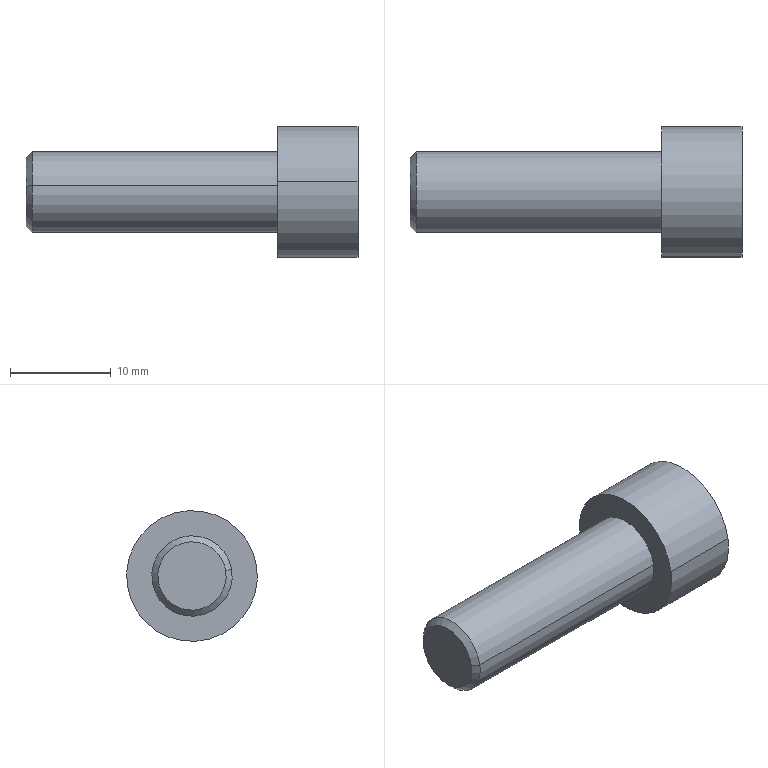Part | SolidWorks | features BaseBody 1 | 1 solid | 16 faces | box 33 x 13 x 13 mm | volume 2189 mm3 | plane 10 | cylinder 4 | cone 2 | commonest cylinder face diameters 8 x2 13 x2
STEP:
#1=CARTESIAN_POINT('',(251.6,-33.855,-27.446));
#2=VERTEX_POINT('',#1);
#3=CARTESIAN_POINT('',(251.6,-27.145,-28.554));
#4=VERTEX_POINT('',#3);
#5=CARTESIAN_POINT('',(251.6,-30.5,-28.));
#6=DIRECTION('',(-1.,0.,0.));
#7=DIRECTION('',(0.,-0.9866,0.1629));
#8=AXIS2_PLACEMENT_3D('',#5,#6,#7);
#9=CIRCLE('',#8,3.4);
#10=EDGE_CURVE('',#2,#4,#9,.T.);
#11=ORIENTED_EDGE('',*,*,#10,.F.);
#12=CARTESIAN_POINT('',(252.2,-34.447,-27.348));
#13=VERTEX_POINT('',#12);
#14=CARTESIAN_POINT('',(251.6,-33.855,-27.446));
#15=DIRECTION('',(0.7071,-0.6977,0.1152));
#16=VECTOR('',#15,1000.);
#17=LINE('',#14,#16);
#18=EDGE_CURVE('',#2,#13,#17,.T.);
#19=ORIENTED_EDGE('',*,*,#18,.T.);
#20=CARTESIAN_POINT('',(252.2,-26.553,-28.652));
#21=VERTEX_POINT('',#20);
#22=CARTESIAN_POINT('',(252.2,-30.5,-28.));
#23=DIRECTION('',(1.,0.,0.));
#24=DIRECTION('',(0.,-0.9866,0.1629));
#25=AXIS2_PLACEMENT_3D('',#22,#23,#24);
#26=CIRCLE('',#25,4.);
#27=EDGE_CURVE('',#21,#13,#26,.T.);
#28=ORIENTED_EDGE('',*,*,#27,.F.);
#29=CARTESIAN_POINT('',(251.6,-27.145,-28.554));
#30=DIRECTION('',(0.7071,0.6977,-0.1152));
#31=VECTOR('',#30,1000.);
#32=LINE('',#29,#31);
#33=EDGE_CURVE('',#4,#21,#32,.T.);
#34=ORIENTED_EDGE('',*,*,#33,.F.);
#35=EDGE_LOOP('',(#11,#19,#28,#34));
#36=FACE_OUTER_BOUND('',#35,.T.);
#37=CARTESIAN_POINT('',(251.6,-30.5,-28.));
#38=DIRECTION('',(1.,0.,0.));
#39=DIRECTION('',(0.,0.9866,-0.1629));
#40=AXIS2_PLACEMENT_3D('',#37,#38,#39);
#41=CONICAL_SURFACE('',#40,3.4,0.7854);
#42=ADVANCED_FACE('',(#36),#41,.T.);
#43=ORIENTED_EDGE('',*,*,#27,.T.);
#44=CARTESIAN_POINT('',(276.6,-34.447,-27.348));
#45=VERTEX_POINT('',#44);
#46=CARTESIAN_POINT('',(251.6,-34.447,-27.348));
#47=DIRECTION('',(1.,0.,0.));
#48=VECTOR('',#47,1000.);
#49=LINE('',#46,#48);
#50=EDGE_CURVE('',#13,#45,#49,.T.);
#51=ORIENTED_EDGE('',*,*,#50,.T.);
#52=CARTESIAN_POINT('',(276.6,-26.553,-28.652));
#53=VERTEX_POINT('',#52);
#54=CARTESIAN_POINT('',(276.6,-30.5,-28.));
#55=DIRECTION('',(-1.,0.,0.));
#56=DIRECTION('',(0.,-0.9866,0.1629));
#57=AXIS2_PLACEMENT_3D('',#54,#55,#56);
#58=CIRCLE('',#57,4.);
#59=EDGE_CURVE('',#45,#53,#58,.T.);
#60=ORIENTED_EDGE('',*,*,#59,.T.);
#61=CARTESIAN_POINT('',(251.6,-26.553,-28.652));
#62=DIRECTION('',(1.,0.,0.));
#63=VECTOR('',#62,1000.);
#64=LINE('',#61,#63);
#65=EDGE_CURVE('',#21,#53,#64,.T.);
#66=ORIENTED_EDGE('',*,*,#65,.F.);
#67=EDGE_LOOP('',(#43,#51,#60,#66));
#68=FACE_OUTER_BOUND('',#67,.T.);
#69=CARTESIAN_POINT('',(251.6,-30.5,-28.));
#70=DIRECTION('',(1.,0.,0.));
#71=DIRECTION('',(0.,0.9866,-0.1629));
#72=AXIS2_PLACEMENT_3D('',#69,#70,#71);
#73=CYLINDRICAL_SURFACE('',#72,4.);
#74=ADVANCED_FACE('',(#68),#73,.T.);
#75=CARTESIAN_POINT('',(276.6,-36.913,-26.941));
#76=VERTEX_POINT('',#75);
#77=CARTESIAN_POINT('',(276.6,-24.087,-29.059));
#78=VERTEX_POINT('',#77);
#79=CARTESIAN_POINT('',(276.6,-30.5,-28.));
#80=DIRECTION('',(-1.,0.,0.));
#81=DIRECTION('',(0.,-0.9866,0.1629));
#82=AXIS2_PLACEMENT_3D('',#79,#80,#81);
#83=CIRCLE('',#82,6.5);
#84=EDGE_CURVE('',#76,#78,#83,.T.);
#85=ORIENTED_EDGE('',*,*,#84,.F.);
#86=CARTESIAN_POINT('',(284.6,-36.913,-26.941));
#87=VERTEX_POINT('',#86);
#88=CARTESIAN_POINT('',(276.6,-36.913,-26.941));
#89=DIRECTION('',(1.,0.,0.));
#90=VECTOR('',#89,1000.);
#91=LINE('',#88,#90);
#92=EDGE_CURVE('',#76,#87,#91,.T.);
#93=ORIENTED_EDGE('',*,*,#92,.T.);
#94=CARTESIAN_POINT('',(284.6,-24.087,-29.059));
#95=VERTEX_POINT('',#94);
#96=CARTESIAN_POINT('',(284.6,-30.5,-28.));
#97=DIRECTION('',(-1.,0.,0.));
#98=DIRECTION('',(0.,-0.9866,0.1629));
#99=AXIS2_PLACEMENT_3D('',#96,#97,#98);
#100=CIRCLE('',#99,6.5);
#101=EDGE_CURVE('',#87,#95,#100,.T.);
#102=ORIENTED_EDGE('',*,*,#101,.T.);
#103=CARTESIAN_POINT('',(276.6,-24.087,-29.059));
#104=DIRECTION('',(1.,0.,0.));
#105=VECTOR('',#104,1000.);
#106=LINE('',#103,#105);
#107=EDGE_CURVE('',#78,#95,#106,.T.);
#108=ORIENTED_EDGE('',*,*,#107,.F.);
#109=EDGE_LOOP('',(#85,#93,#102,#108));
#110=FACE_OUTER_BOUND('',#109,.T.);
#111=CARTESIAN_POINT('',(276.6,-30.5,-28.));
#112=DIRECTION('',(1.,0.,0.));
#113=DIRECTION('',(0.,0.9866,-0.1629));
#114=AXIS2_PLACEMENT_3D('',#111,#112,#113);
#115=CYLINDRICAL_SURFACE('',#114,6.5);
#116=ADVANCED_FACE('',(#110),#115,.T.);
#117=CARTESIAN_POINT('',(276.6,-30.5,-28.));
#118=DIRECTION('',(-1.,0.,0.));
#119=DIRECTION('',(0.,-0.9866,0.1629));
#120=AXIS2_PLACEMENT_3D('',#117,#118,#119);
#121=CIRCLE('',#120,6.5);
#122=EDGE_CURVE('',#78,#76,#121,.T.);
#123=ORIENTED_EDGE('',*,*,#122,.T.);
#124=ORIENTED_EDGE('',*,*,#84,.T.);
#125=EDGE_LOOP('',(#123,#124));
#126=FACE_OUTER_BOUND('',#125,.T.);
#127=CARTESIAN_POINT('',(276.6,-30.5,-28.));
#128=DIRECTION('',(-1.,0.,0.));
#129=DIRECTION('',(0.,-0.9866,0.1629));
#130=AXIS2_PLACEMENT_3D('',#127,#128,#129);
#131=CIRCLE('',#130,4.);
#132=EDGE_CURVE('',#53,#45,#131,.T.);
#133=ORIENTED_EDGE('',*,*,#132,.F.);
#134=ORIENTED_EDGE('',*,*,#59,.F.);
#135=EDGE_LOOP('',(#133,#134));
#136=FACE_BOUND('',#135,.T.);
#137=CARTESIAN_POINT('',(276.6,-30.5,-28.));
#138=DIRECTION('',(-1.,0.,0.));
#139=DIRECTION('',(0.,-0.9866,0.1629));
#140=AXIS2_PLACEMENT_3D('',#137,#138,#139);
#141=PLANE('',#140);
#142=ADVANCED_FACE('',(#126,#136),#141,.T.);
#143=ORIENTED_EDGE('',*,*,#92,.F.);
#144=ORIENTED_EDGE('',*,*,#122,.F.);
#145=ORIENTED_EDGE('',*,*,#107,.T.);
#146=CARTESIAN_POINT('',(284.6,-30.5,-28.));
#147=DIRECTION('',(-1.,0.,0.));
#148=DIRECTION('',(0.,-0.9866,0.1629));
#149=AXIS2_PLACEMENT_3D('',#146,#147,#148);
#150=CIRCLE('',#149,6.5);
#151=EDGE_CURVE('',#95,#87,#150,.T.);
#152=ORIENTED_EDGE('',*,*,#151,.T.);
#153=EDGE_LOOP('',(#143,#144,#145,#152));
#154=FACE_OUTER_BOUND('',#153,.T.);
#155=CARTESIAN_POINT('',(276.6,-30.5,-28.));
#156=DIRECTION('',(1.,0.,0.));
#157=DIRECTION('',(0.,0.9866,-0.1629));
#158=AXIS2_PLACEMENT_3D('',#155,#156,#157);
#159=CYLINDRICAL_SURFACE('',#158,6.5);
#160=ADVANCED_FACE('',(#154),#159,.T.);
#161=CARTESIAN_POINT('',(284.6,-33.178,-25.802));
#162=VERTEX_POINT('',#161);
#163=CARTESIAN_POINT('',(284.6,-33.742,-29.22));
#164=VERTEX_POINT('',#163);
#165=CARTESIAN_POINT('',(284.6,-33.178,-25.802));
#166=DIRECTION('',(0.,-0.1629,-0.9866));
#167=VECTOR('',#166,1000.);
#168=LINE('',#165,#167);
#169=EDGE_CURVE('',#162,#164,#168,.T.);
#170=ORIENTED_EDGE('',*,*,#169,.F.);
#171=CARTESIAN_POINT('',(284.6,-29.936,-24.582));
#172=VERTEX_POINT('',#171);
#173=CARTESIAN_POINT('',(284.6,-29.936,-24.582));
#174=DIRECTION('',(0.,-0.9359,-0.3522));
#175=VECTOR('',#174,1000.);
#176=LINE('',#173,#175);
#177=EDGE_CURVE('',#172,#162,#176,.T.);
#178=ORIENTED_EDGE('',*,*,#177,.F.);
#179=CARTESIAN_POINT('',(284.6,-27.258,-26.78));
#180=VERTEX_POINT('',#179);
#181=CARTESIAN_POINT('',(284.6,-29.936,-24.582));
#182=DIRECTION('',(0.,-0.773,0.6344));
#183=VECTOR('',#182,1000.);
#184=LINE('',#181,#183);
#185=EDGE_CURVE('',#180,#172,#184,.T.);
#186=ORIENTED_EDGE('',*,*,#185,.F.);
#187=CARTESIAN_POINT('',(284.6,-27.822,-30.198));
#188=VERTEX_POINT('',#187);
#189=CARTESIAN_POINT('',(284.6,-27.258,-26.78));
#190=DIRECTION('',(0.,0.1629,0.9866));
#191=VECTOR('',#190,1000.);
#192=LINE('',#189,#191);
#193=EDGE_CURVE('',#188,#180,#192,.T.);
#194=ORIENTED_EDGE('',*,*,#193,.F.);
#195=CARTESIAN_POINT('',(284.6,-31.064,-31.418));
#196=VERTEX_POINT('',#195);
#197=CARTESIAN_POINT('',(284.6,-31.064,-31.418));
#198=DIRECTION('',(0.,0.9359,0.3522));
#199=VECTOR('',#198,1000.);
#200=LINE('',#197,#199);
#201=EDGE_CURVE('',#196,#188,#200,.T.);
#202=ORIENTED_EDGE('',*,*,#201,.F.);
#203=CARTESIAN_POINT('',(284.6,-31.064,-31.418));
#204=DIRECTION('',(0.,0.773,-0.6344));
#205=VECTOR('',#204,1000.);
#206=LINE('',#203,#205);
#207=EDGE_CURVE('',#164,#196,#206,.T.);
#208=ORIENTED_EDGE('',*,*,#207,.F.);
#209=EDGE_LOOP('',(#170,#178,#186,#194,#202,#208));
#210=FACE_BOUND('',#209,.T.);
#211=ORIENTED_EDGE('',*,*,#151,.F.);
#212=ORIENTED_EDGE('',*,*,#101,.F.);
#213=EDGE_LOOP('',(#211,#212));
#214=FACE_OUTER_BOUND('',#213,.T.);
#215=CARTESIAN_POINT('',(284.6,-30.5,-28.));
#216=DIRECTION('',(-1.,0.,0.));
#217=DIRECTION('',(0.,-0.9866,0.1629));
#218=AXIS2_PLACEMENT_3D('',#215,#216,#217);
#219=PLANE('',#218);
#220=ADVANCED_FACE('',(#210,#214),#219,.F.);
#221=ORIENTED_EDGE('',*,*,#50,.F.);
#222=CARTESIAN_POINT('',(252.2,-30.5,-28.));
#223=DIRECTION('',(1.,0.,0.));
#224=DIRECTION('',(0.,-0.9866,0.1629));
#225=AXIS2_PLACEMENT_3D('',#222,#223,#224);
#226=CIRCLE('',#225,4.);
#227=EDGE_CURVE('',#13,#21,#226,.T.);
#228=ORIENTED_EDGE('',*,*,#227,.T.);
#229=ORIENTED_EDGE('',*,*,#65,.T.);
#230=ORIENTED_EDGE('',*,*,#132,.T.);
#231=EDGE_LOOP('',(#221,#228,#229,#230));
#232=FACE_OUTER_BOUND('',#231,.T.);
#233=CARTESIAN_POINT('',(251.6,-30.5,-28.));
#234=DIRECTION('',(1.,0.,0.));
#235=DIRECTION('',(0.,0.9866,-0.1629));
#236=AXIS2_PLACEMENT_3D('',#233,#234,#235);
#237=CYLINDRICAL_SURFACE('',#236,4.);
#238=ADVANCED_FACE('',(#232),#237,.T.);
#239=CARTESIAN_POINT('',(251.6,-30.5,-28.));
#240=DIRECTION('',(-1.,0.,0.));
#241=DIRECTION('',(0.,-0.9866,0.1629));
#242=AXIS2_PLACEMENT_3D('',#239,#240,#241);
#243=CIRCLE('',#242,3.4);
#244=EDGE_CURVE('',#4,#2,#243,.T.);
#245=ORIENTED_EDGE('',*,*,#244,.T.);
#246=ORIENTED_EDGE('',*,*,#10,.T.);
#247=EDGE_LOOP('',(#245,#246));
#248=FACE_OUTER_BOUND('',#247,.T.);
#249=CARTESIAN_POINT('',(251.6,-30.5,-28.));
#250=DIRECTION('',(-1.,0.,0.));
#251=DIRECTION('',(0.,-0.9866,0.1629));
#252=AXIS2_PLACEMENT_3D('',#249,#250,#251);
#253=PLANE('',#252);
#254=ADVANCED_FACE('',(#248),#253,.T.);
#255=ORIENTED_EDGE('',*,*,#177,.T.);
#256=CARTESIAN_POINT('',(280.6,-33.178,-25.802));
#257=VERTEX_POINT('',#256);
#258=CARTESIAN_POINT('',(280.6,-33.178,-25.802));
#259=DIRECTION('',(1.,0.,0.));
#260=VECTOR('',#259,1000.);
#261=LINE('',#258,#260);
#262=EDGE_CURVE('',#257,#162,#261,.T.);
#263=ORIENTED_EDGE('',*,*,#262,.F.);
#264=CARTESIAN_POINT('',(280.6,-29.936,-24.582));
#265=VERTEX_POINT('',#264);
#266=CARTESIAN_POINT('',(280.6,-29.936,-24.582));
#267=DIRECTION('',(0.,-0.9359,-0.3522));
#268=VECTOR('',#267,1000.);
#269=LINE('',#266,#268);
#270=EDGE_CURVE('',#265,#257,#269,.T.);
#271=ORIENTED_EDGE('',*,*,#270,.F.);
#272=CARTESIAN_POINT('',(280.6,-29.936,-24.582));
#273=DIRECTION('',(1.,0.,0.));
#274=VECTOR('',#273,1000.);
#275=LINE('',#272,#274);
#276=EDGE_CURVE('',#265,#172,#275,.T.);
#277=ORIENTED_EDGE('',*,*,#276,.T.);
#278=EDGE_LOOP('',(#255,#263,#271,#277));
#279=FACE_OUTER_BOUND('',#278,.T.);
#280=CARTESIAN_POINT('',(280.6,-29.936,-24.582));
#281=DIRECTION('',(0.,-0.3522,0.9359));
#282=DIRECTION('',(0.,0.9359,0.3522));
#283=AXIS2_PLACEMENT_3D('',#280,#281,#282);
#284=PLANE('',#283);
#285=ADVANCED_FACE('',(#279),#284,.F.);
#286=ORIENTED_EDGE('',*,*,#185,.T.);
#287=ORIENTED_EDGE('',*,*,#276,.F.);
#288=CARTESIAN_POINT('',(280.6,-27.258,-26.78));
#289=VERTEX_POINT('',#288);
#290=CARTESIAN_POINT('',(280.6,-29.936,-24.582));
#291=DIRECTION('',(0.,-0.773,0.6344));
#292=VECTOR('',#291,1000.);
#293=LINE('',#290,#292);
#294=EDGE_CURVE('',#289,#265,#293,.T.);
#295=ORIENTED_EDGE('',*,*,#294,.F.);
#296=CARTESIAN_POINT('',(280.6,-27.258,-26.78));
#297=DIRECTION('',(1.,0.,0.));
#298=VECTOR('',#297,1000.);
#299=LINE('',#296,#298);
#300=EDGE_CURVE('',#289,#180,#299,.T.);
#301=ORIENTED_EDGE('',*,*,#300,.T.);
#302=EDGE_LOOP('',(#286,#287,#295,#301));
#303=FACE_OUTER_BOUND('',#302,.T.);
#304=CARTESIAN_POINT('',(280.6,-29.936,-24.582));
#305=DIRECTION('',(0.,0.6344,0.773));
#306=DIRECTION('',(0.,0.773,-0.6344));
#307=AXIS2_PLACEMENT_3D('',#304,#305,#306);
#308=PLANE('',#307);
#309=ADVANCED_FACE('',(#303),#308,.F.);
#310=ORIENTED_EDGE('',*,*,#193,.T.);
#311=ORIENTED_EDGE('',*,*,#300,.F.);
#312=CARTESIAN_POINT('',(280.6,-27.822,-30.198));
#313=VERTEX_POINT('',#312);
#314=CARTESIAN_POINT('',(280.6,-27.258,-26.78));
#315=DIRECTION('',(0.,0.1629,0.9866));
#316=VECTOR('',#315,1000.);
#317=LINE('',#314,#316);
#318=EDGE_CURVE('',#313,#289,#317,.T.);
#319=ORIENTED_EDGE('',*,*,#318,.F.);
#320=CARTESIAN_POINT('',(280.6,-27.822,-30.198));
#321=DIRECTION('',(1.,0.,0.));
#322=VECTOR('',#321,1000.);
#323=LINE('',#320,#322);
#324=EDGE_CURVE('',#313,#188,#323,.T.);
#325=ORIENTED_EDGE('',*,*,#324,.T.);
#326=EDGE_LOOP('',(#310,#311,#319,#325));
#327=FACE_OUTER_BOUND('',#326,.T.);
#328=CARTESIAN_POINT('',(280.6,-27.258,-26.78));
#329=DIRECTION('',(0.,0.9866,-0.1629));
#330=DIRECTION('',(-1.,0.,0.));
#331=AXIS2_PLACEMENT_3D('',#328,#329,#330);
#332=PLANE('',#331);
#333=ADVANCED_FACE('',(#327),#332,.F.);
#334=ORIENTED_EDGE('',*,*,#201,.T.);
#335=ORIENTED_EDGE('',*,*,#324,.F.);
#336=CARTESIAN_POINT('',(280.6,-31.064,-31.418));
#337=VERTEX_POINT('',#336);
#338=CARTESIAN_POINT('',(280.6,-31.064,-31.418));
#339=DIRECTION('',(0.,0.9359,0.3522));
#340=VECTOR('',#339,1000.);
#341=LINE('',#338,#340);
#342=EDGE_CURVE('',#337,#313,#341,.T.);
#343=ORIENTED_EDGE('',*,*,#342,.F.);
#344=CARTESIAN_POINT('',(280.6,-31.064,-31.418));
#345=DIRECTION('',(1.,0.,0.));
#346=VECTOR('',#345,1000.);
#347=LINE('',#344,#346);
#348=EDGE_CURVE('',#337,#196,#347,.T.);
#349=ORIENTED_EDGE('',*,*,#348,.T.);
#350=EDGE_LOOP('',(#334,#335,#343,#349));
#351=FACE_OUTER_BOUND('',#350,.T.);
#352=CARTESIAN_POINT('',(280.6,-31.064,-31.418));
#353=DIRECTION('',(0.,0.3522,-0.9359));
#354=DIRECTION('',(0.,-0.9359,-0.3522));
#355=AXIS2_PLACEMENT_3D('',#352,#353,#354);
#356=PLANE('',#355);
#357=ADVANCED_FACE('',(#351),#356,.F.);
#358=ORIENTED_EDGE('',*,*,#207,.T.);
#359=ORIENTED_EDGE('',*,*,#348,.F.);
#360=CARTESIAN_POINT('',(280.6,-33.742,-29.22));
#361=VERTEX_POINT('',#360);
#362=CARTESIAN_POINT('',(280.6,-31.064,-31.418));
#363=DIRECTION('',(0.,0.773,-0.6344));
#364=VECTOR('',#363,1000.);
#365=LINE('',#362,#364);
#366=EDGE_CURVE('',#361,#337,#365,.T.);
#367=ORIENTED_EDGE('',*,*,#366,.F.);
#368=CARTESIAN_POINT('',(280.6,-33.742,-29.22));
#369=DIRECTION('',(1.,0.,0.));
#370=VECTOR('',#369,1000.);
#371=LINE('',#368,#370);
#372=EDGE_CURVE('',#361,#164,#371,.T.);
#373=ORIENTED_EDGE('',*,*,#372,.T.);
#374=EDGE_LOOP('',(#358,#359,#367,#373));
#375=FACE_OUTER_BOUND('',#374,.T.);
#376=CARTESIAN_POINT('',(280.6,-31.064,-31.418));
#377=DIRECTION('',(0.,-0.6344,-0.773));
#378=DIRECTION('',(0.,-0.773,0.6344));
#379=AXIS2_PLACEMENT_3D('',#376,#377,#378);
#380=PLANE('',#379);
#381=ADVANCED_FACE('',(#375),#380,.F.);
#382=ORIENTED_EDGE('',*,*,#169,.T.);
#383=ORIENTED_EDGE('',*,*,#372,.F.);
#384=CARTESIAN_POINT('',(280.6,-33.178,-25.802));
#385=DIRECTION('',(0.,-0.1629,-0.9866));
#386=VECTOR('',#385,1000.);
#387=LINE('',#384,#386);
#388=EDGE_CURVE('',#257,#361,#387,.T.);
#389=ORIENTED_EDGE('',*,*,#388,.F.);
#390=ORIENTED_EDGE('',*,*,#262,.T.);
#391=EDGE_LOOP('',(#382,#383,#389,#390));
#392=FACE_OUTER_BOUND('',#391,.T.);
#393=CARTESIAN_POINT('',(280.6,-33.178,-25.802));
#394=DIRECTION('',(0.,-0.9866,0.1629));
#395=DIRECTION('',(1.,0.,0.));
#396=AXIS2_PLACEMENT_3D('',#393,#394,#395);
#397=PLANE('',#396);
#398=ADVANCED_FACE('',(#392),#397,.F.);
#399=ORIENTED_EDGE('',*,*,#270,.T.);
#400=ORIENTED_EDGE('',*,*,#388,.T.);
#401=ORIENTED_EDGE('',*,*,#366,.T.);
#402=ORIENTED_EDGE('',*,*,#342,.T.);
#403=ORIENTED_EDGE('',*,*,#318,.T.);
#404=ORIENTED_EDGE('',*,*,#294,.T.);
#405=EDGE_LOOP('',(#399,#400,#401,#402,#403,#404));
#406=FACE_OUTER_BOUND('',#405,.T.);
#407=CARTESIAN_POINT('',(280.6,-36.42,-27.022));
#408=DIRECTION('',(-1.,0.,0.));
#409=DIRECTION('',(0.,-0.9866,0.1629));
#410=AXIS2_PLACEMENT_3D('',#407,#408,#409);
#411=PLANE('',#410);
#412=ADVANCED_FACE('',(#406),#411,.F.);
#413=ORIENTED_EDGE('',*,*,#18,.F.);
#414=ORIENTED_EDGE('',*,*,#244,.F.);
#415=ORIENTED_EDGE('',*,*,#33,.T.);
#416=ORIENTED_EDGE('',*,*,#227,.F.);
#417=EDGE_LOOP('',(#413,#414,#415,#416));
#418=FACE_OUTER_BOUND('',#417,.T.);
#419=CARTESIAN_POINT('',(251.6,-30.5,-28.));
#420=DIRECTION('',(1.,0.,0.));
#421=DIRECTION('',(0.,0.9866,-0.1629));
#422=AXIS2_PLACEMENT_3D('',#419,#420,#421);
#423=CONICAL_SURFACE('',#422,3.4,0.7854);
#424=ADVANCED_FACE('',(#418),#423,.T.);
#425=CLOSED_SHELL('',(#42,#74,#116,#142,#160,#220,#238,#254,#285,#309,#333,#357,#381,#398,#412,#424));
#426=MANIFOLD_SOLID_BREP('',#425);
#427=CARTESIAN_POINT('',(0.,0.,0.));
#428=DIRECTION('',(0.,0.,1.));
#429=DIRECTION('',(1.,0.,0.));
#430=AXIS2_PLACEMENT_3D('',#427,#428,#429);
#431=(LENGTH_UNIT()NAMED_UNIT(*)SI_UNIT(.MILLI.,.METRE.));
#432=UNCERTAINTY_MEASURE_WITH_UNIT(LENGTH_MEASURE(0.00001),#431,'','');
#433=(NAMED_UNIT(*)PLANE_ANGLE_UNIT()SI_UNIT($,.RADIAN.));
#434=(NAMED_UNIT(*)SI_UNIT($,.STERADIAN.)SOLID_ANGLE_UNIT());
#435=(GEOMETRIC_REPRESENTATION_CONTEXT(3)GLOBAL_UNCERTAINTY_ASSIGNED_CONTEXT((#432))GLOBAL_UNIT_ASSIGNED_CONTEXT((#431,#433,#434))REPRESENTATION_CONTEXT('',''));
#436=ADVANCED_BREP_SHAPE_REPRESENTATION('',(#426,#430),#435);